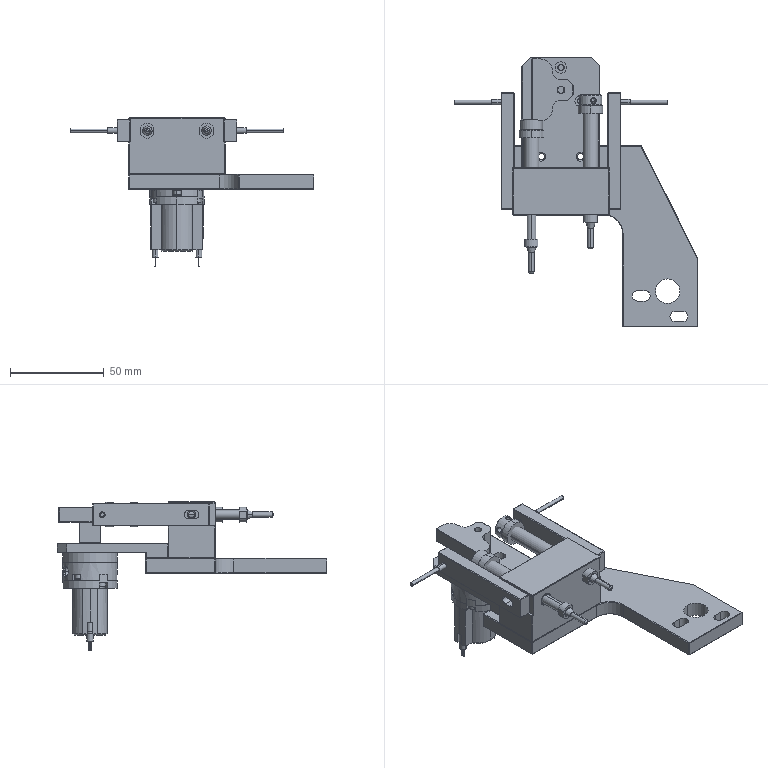Part | NX | 27 solids | 1058 faces | box 129.5 x 143.5 x 79.237 mm | volume 128433 mm3 | cylinder 412 | plane 360 | cone 146 | torus 96 | sphere 36 | spline 8 | commonest cylinder face diameters 0.4 x114 5 x49 4 x40 3 x22 3.3 x20 7 x20